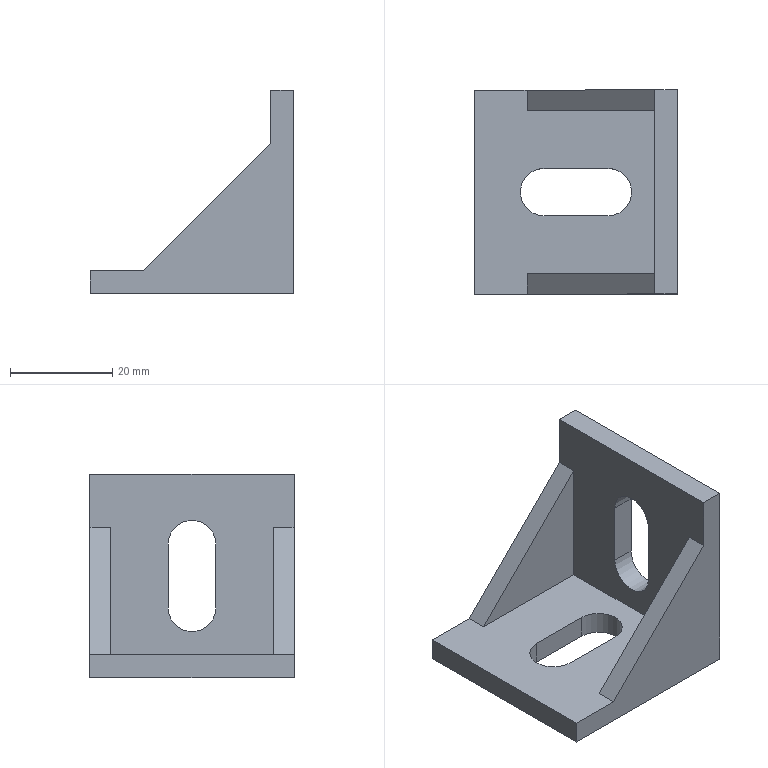Part | STEP file | 40x40 angle bracket | 1 solid | 20 faces | box 39.8 x 40 x 39.8 mm | volume 14360 mm3 | plane 16 | cylinder 4 | commonest cylinder face diameters 9.3 x4
STEP:
#1=CARTESIAN_POINT('',(0.,0.,0.));
#2=DIRECTION('',(0.,0.,1.));
#3=DIRECTION('',(1.,0.,0.));
#4=AXIS2_PLACEMENT_3D('',#1,#2,#3);
#5=CARTESIAN_POINT('',(400.35,-329.65,4.5));
#6=VERTEX_POINT('',#5);
#7=CARTESIAN_POINT('',(412.85,-329.65,4.5));
#8=VERTEX_POINT('',#7);
#9=CARTESIAN_POINT('',(386.7,-329.65,4.5));
#10=DIRECTION('',(1.,0.,0.));
#11=VECTOR('',#10,1.);
#12=LINE('',#9,#11);
#13=CARTESIAN_POINT('',(400.35,-329.65,44.5));
#14=DIRECTION('',(0.,-1.,0.));
#15=DIRECTION('',(0.,0.,1.));
#16=AXIS2_PLACEMENT_3D('',#13,#14,#15);
#17=PLANE('',#16);
#18=CARTESIAN_POINT('',(-40.,13.65));
#19=DIRECTION('',(0.,-1.));
#20=VECTOR('',#19,1.);
#21=LINE('',#18,#20);
#22=(GEOMETRIC_REPRESENTATION_CONTEXT(2)PARAMETRIC_REPRESENTATION_CONTEXT()REPRESENTATION_CONTEXT('',''));
#23=DEFINITIONAL_REPRESENTATION('',(#21),#22);
#24=PCURVE('',#17,#23);
#25=CARTESIAN_POINT('',(386.7,-305.,4.5));
#26=DIRECTION('',(0.,0.,1.));
#27=DIRECTION('',(1.,0.,0.));
#28=AXIS2_PLACEMENT_3D('',#25,#26,#27);
#29=PLANE('',#28);
#30=CARTESIAN_POINT('',(0.,-24.65));
#31=DIRECTION('',(1.,0.));
#32=VECTOR('',#31,1.);
#33=LINE('',#30,#32);
#34=(GEOMETRIC_REPRESENTATION_CONTEXT(2)PARAMETRIC_REPRESENTATION_CONTEXT()REPRESENTATION_CONTEXT('',''));
#35=DEFINITIONAL_REPRESENTATION('',(#33),#34);
#36=PCURVE('',#29,#35);
#37=SURFACE_CURVE('',#12,(#24,#36),.PCURVE_S1.);
#38=EDGE_CURVE('',#6,#8,#37,.T.);
#39=ORIENTED_EDGE('',*,*,#38,.T.);
#40=CARTESIAN_POINT('',(412.85,-329.65,0.));
#41=VERTEX_POINT('',#40);
#42=CARTESIAN_POINT('',(412.85,-329.65,44.5));
#43=DIRECTION('',(0.,0.,-1.));
#44=VECTOR('',#43,1.);
#45=LINE('',#42,#44);
#46=CARTESIAN_POINT('',(0.,-12.5));
#47=DIRECTION('',(-1.,0.));
#48=VECTOR('',#47,1.);
#49=LINE('',#46,#48);
#50=(GEOMETRIC_REPRESENTATION_CONTEXT(2)PARAMETRIC_REPRESENTATION_CONTEXT()REPRESENTATION_CONTEXT('',''));
#51=DEFINITIONAL_REPRESENTATION('',(#49),#50);
#52=PCURVE('',#17,#51);
#53=CARTESIAN_POINT('',(412.85,-325.,44.5));
#54=DIRECTION('',(0.,0.,-1.));
#55=DIRECTION('',(-1.,0.,0.));
#56=AXIS2_PLACEMENT_3D('',#53,#54,#55);
#57=CYLINDRICAL_SURFACE('',#56,4.65);
#58=CARTESIAN_POINT('',(4.712,0.));
#59=DIRECTION('',(0.,1.));
#60=VECTOR('',#59,1.);
#61=LINE('',#58,#60);
#62=(GEOMETRIC_REPRESENTATION_CONTEXT(2)PARAMETRIC_REPRESENTATION_CONTEXT()REPRESENTATION_CONTEXT('',''));
#63=DEFINITIONAL_REPRESENTATION('',(#61),#62);
#64=PCURVE('',#57,#63);
#65=SURFACE_CURVE('',#45,(#52,#64),.PCURVE_S1.);
#66=EDGE_CURVE('',#8,#41,#65,.T.);
#67=ORIENTED_EDGE('',*,*,#66,.T.);
#68=CARTESIAN_POINT('',(400.35,-329.65,0.));
#69=VERTEX_POINT('',#68);
#70=CARTESIAN_POINT('',(426.5,-329.65,0.));
#71=DIRECTION('',(-1.,0.,0.));
#72=VECTOR('',#71,1.);
#73=LINE('',#70,#72);
#74=CARTESIAN_POINT('',(-44.5,-26.15));
#75=DIRECTION('',(0.,1.));
#76=VECTOR('',#75,1.);
#77=LINE('',#74,#76);
#78=(GEOMETRIC_REPRESENTATION_CONTEXT(2)PARAMETRIC_REPRESENTATION_CONTEXT()REPRESENTATION_CONTEXT('',''));
#79=DEFINITIONAL_REPRESENTATION('',(#77),#78);
#80=PCURVE('',#17,#79);
#81=CARTESIAN_POINT('',(426.5,-305.,0.));
#82=DIRECTION('',(0.,0.,-1.));
#83=DIRECTION('',(-1.,0.,0.));
#84=AXIS2_PLACEMENT_3D('',#81,#82,#83);
#85=PLANE('',#84);
#86=CARTESIAN_POINT('',(0.,-24.65));
#87=DIRECTION('',(1.,0.));
#88=VECTOR('',#87,1.);
#89=LINE('',#86,#88);
#90=(GEOMETRIC_REPRESENTATION_CONTEXT(2)PARAMETRIC_REPRESENTATION_CONTEXT()REPRESENTATION_CONTEXT('',''));
#91=DEFINITIONAL_REPRESENTATION('',(#89),#90);
#92=PCURVE('',#85,#91);
#93=SURFACE_CURVE('',#73,(#80,#92),.PCURVE_S1.);
#94=EDGE_CURVE('',#41,#69,#93,.T.);
#95=ORIENTED_EDGE('',*,*,#94,.T.);
#96=CARTESIAN_POINT('',(400.35,-329.65,44.5));
#97=DIRECTION('',(0.,0.,-1.));
#98=VECTOR('',#97,1.);
#99=LINE('',#96,#98);
#100=CARTESIAN_POINT('',(0.,0.));
#101=DIRECTION('',(-1.,0.));
#102=VECTOR('',#101,1.);
#103=LINE('',#100,#102);
#104=(GEOMETRIC_REPRESENTATION_CONTEXT(2)PARAMETRIC_REPRESENTATION_CONTEXT()REPRESENTATION_CONTEXT('',''));
#105=DEFINITIONAL_REPRESENTATION('',(#103),#104);
#106=PCURVE('',#17,#105);
#107=CARTESIAN_POINT('',(400.35,-325.,44.5));
#108=DIRECTION('',(0.,0.,-1.));
#109=DIRECTION('',(-1.,0.,0.));
#110=AXIS2_PLACEMENT_3D('',#107,#108,#109);
#111=CYLINDRICAL_SURFACE('',#110,4.65);
#112=CARTESIAN_POINT('',(-1.571,0.));
#113=DIRECTION('',(0.,1.));
#114=VECTOR('',#113,1.);
#115=LINE('',#112,#114);
#116=(GEOMETRIC_REPRESENTATION_CONTEXT(2)PARAMETRIC_REPRESENTATION_CONTEXT()REPRESENTATION_CONTEXT('',''));
#117=DEFINITIONAL_REPRESENTATION('',(#115),#116);
#118=PCURVE('',#111,#117);
#119=SURFACE_CURVE('',#99,(#106,#118),.PCURVE_S1.);
#120=EDGE_CURVE('',#6,#69,#119,.T.);
#121=ORIENTED_EDGE('',*,*,#120,.F.);
#122=EDGE_LOOP('',(#39,#67,#95,#121));
#123=FACE_BOUND('',#122,.T.);
#124=ADVANCED_FACE('',(#123),#17,.F.);
#125=ORIENTED_EDGE('',*,*,#66,.T.);
#126=CARTESIAN_POINT('',(412.85,-320.35,0.));
#127=VERTEX_POINT('',#126);
#128=CARTESIAN_POINT('',(412.85,-325.,0.));
#129=DIRECTION('',(0.,0.,-1.));
#130=DIRECTION('',(-1.,0.,0.));
#131=AXIS2_PLACEMENT_3D('',#128,#129,#130);
#132=CIRCLE('',#131,4.65);
#133=CARTESIAN_POINT('',(0.,44.5));
#134=DIRECTION('',(1.,0.));
#135=VECTOR('',#134,1.);
#136=LINE('',#133,#135);
#137=(GEOMETRIC_REPRESENTATION_CONTEXT(2)PARAMETRIC_REPRESENTATION_CONTEXT()REPRESENTATION_CONTEXT('',''));
#138=DEFINITIONAL_REPRESENTATION('',(#136),#137);
#139=PCURVE('',#57,#138);
#140=CARTESIAN_POINT('',(13.65,-20.));
#141=DIRECTION('',(1.,0.));
#142=AXIS2_PLACEMENT_2D('',#140,#141);
#143=CIRCLE('',#142,4.65);
#144=(GEOMETRIC_REPRESENTATION_CONTEXT(2)PARAMETRIC_REPRESENTATION_CONTEXT()REPRESENTATION_CONTEXT('',''));
#145=DEFINITIONAL_REPRESENTATION('',(#143),#144);
#146=PCURVE('',#85,#145);
#147=SURFACE_CURVE('',#132,(#139,#146),.PCURVE_S1.);
#148=EDGE_CURVE('',#127,#41,#147,.T.);
#149=ORIENTED_EDGE('',*,*,#148,.F.);
#150=CARTESIAN_POINT('',(412.85,-320.35,4.5));
#151=VERTEX_POINT('',#150);
#152=CARTESIAN_POINT('',(412.85,-320.35,44.5));
#153=DIRECTION('',(0.,0.,-1.));
#154=VECTOR('',#153,1.);
#155=LINE('',#152,#154);
#156=CARTESIAN_POINT('',(1.571,0.));
#157=DIRECTION('',(0.,1.));
#158=VECTOR('',#157,1.);
#159=LINE('',#156,#158);
#160=(GEOMETRIC_REPRESENTATION_CONTEXT(2)PARAMETRIC_REPRESENTATION_CONTEXT()REPRESENTATION_CONTEXT('',''));
#161=DEFINITIONAL_REPRESENTATION('',(#159),#160);
#162=PCURVE('',#57,#161);
#163=CARTESIAN_POINT('',(412.85,-320.35,44.5));
#164=DIRECTION('',(0.,1.,0.));
#165=DIRECTION('',(0.,0.,-1.));
#166=AXIS2_PLACEMENT_3D('',#163,#164,#165);
#167=PLANE('',#166);
#168=CARTESIAN_POINT('',(0.,0.));
#169=DIRECTION('',(1.,0.));
#170=VECTOR('',#169,1.);
#171=LINE('',#168,#170);
#172=(GEOMETRIC_REPRESENTATION_CONTEXT(2)PARAMETRIC_REPRESENTATION_CONTEXT()REPRESENTATION_CONTEXT('',''));
#173=DEFINITIONAL_REPRESENTATION('',(#171),#172);
#174=PCURVE('',#167,#173);
#175=SURFACE_CURVE('',#155,(#162,#174),.PCURVE_S1.);
#176=EDGE_CURVE('',#151,#127,#175,.T.);
#177=ORIENTED_EDGE('',*,*,#176,.F.);
#178=CARTESIAN_POINT('',(412.85,-325.,4.5));
#179=DIRECTION('',(0.,0.,1.));
#180=DIRECTION('',(1.,0.,0.));
#181=AXIS2_PLACEMENT_3D('',#178,#179,#180);
#182=CIRCLE('',#181,4.65);
#183=CARTESIAN_POINT('',(9.425,40.));
#184=DIRECTION('',(-1.,0.));
#185=VECTOR('',#184,1.);
#186=LINE('',#183,#185);
#187=(GEOMETRIC_REPRESENTATION_CONTEXT(2)PARAMETRIC_REPRESENTATION_CONTEXT()REPRESENTATION_CONTEXT('',''));
#188=DEFINITIONAL_REPRESENTATION('',(#186),#187);
#189=PCURVE('',#57,#188);
#190=CARTESIAN_POINT('',(26.15,-20.));
#191=DIRECTION('',(1.,0.));
#192=AXIS2_PLACEMENT_2D('',#190,#191);
#193=CIRCLE('',#192,4.65);
#194=(GEOMETRIC_REPRESENTATION_CONTEXT(2)PARAMETRIC_REPRESENTATION_CONTEXT()REPRESENTATION_CONTEXT('',''));
#195=DEFINITIONAL_REPRESENTATION('',(#193),#194);
#196=PCURVE('',#29,#195);
#197=SURFACE_CURVE('',#182,(#189,#196),.PCURVE_S1.);
#198=EDGE_CURVE('',#8,#151,#197,.T.);
#199=ORIENTED_EDGE('',*,*,#198,.F.);
#200=EDGE_LOOP('',(#125,#149,#177,#199));
#201=FACE_BOUND('',#200,.F.);
#202=ADVANCED_FACE('',(#201),#57,.F.);
#203=CARTESIAN_POINT('',(400.35,-320.35,4.5));
#204=VERTEX_POINT('',#203);
#205=CARTESIAN_POINT('',(386.7,-320.35,4.5));
#206=DIRECTION('',(-1.,0.,0.));
#207=VECTOR('',#206,1.);
#208=LINE('',#205,#207);
#209=CARTESIAN_POINT('',(40.,26.15));
#210=DIRECTION('',(0.,1.));
#211=VECTOR('',#210,1.);
#212=LINE('',#209,#211);
#213=(GEOMETRIC_REPRESENTATION_CONTEXT(2)PARAMETRIC_REPRESENTATION_CONTEXT()REPRESENTATION_CONTEXT('',''));
#214=DEFINITIONAL_REPRESENTATION('',(#212),#213);
#215=PCURVE('',#167,#214);
#216=CARTESIAN_POINT('',(0.,-15.35));
#217=DIRECTION('',(-1.,0.));
#218=VECTOR('',#217,1.);
#219=LINE('',#216,#218);
#220=(GEOMETRIC_REPRESENTATION_CONTEXT(2)PARAMETRIC_REPRESENTATION_CONTEXT()REPRESENTATION_CONTEXT('',''));
#221=DEFINITIONAL_REPRESENTATION('',(#219),#220);
#222=PCURVE('',#29,#221);
#223=SURFACE_CURVE('',#208,(#215,#222),.PCURVE_S1.);
#224=EDGE_CURVE('',#151,#204,#223,.T.);
#225=ORIENTED_EDGE('',*,*,#224,.T.);
#226=CARTESIAN_POINT('',(400.35,-320.35,0.));
#227=VERTEX_POINT('',#226);
#228=CARTESIAN_POINT('',(400.35,-320.35,44.5));
#229=DIRECTION('',(0.,0.,-1.));
#230=VECTOR('',#229,1.);
#231=LINE('',#228,#230);
#232=CARTESIAN_POINT('',(0.,12.5));
#233=DIRECTION('',(1.,0.));
#234=VECTOR('',#233,1.);
#235=LINE('',#232,#234);
#236=(GEOMETRIC_REPRESENTATION_CONTEXT(2)PARAMETRIC_REPRESENTATION_CONTEXT()REPRESENTATION_CONTEXT('',''));
#237=DEFINITIONAL_REPRESENTATION('',(#235),#236);
#238=PCURVE('',#167,#237);
#239=CARTESIAN_POINT('',(1.571,0.));
#240=DIRECTION('',(0.,1.));
#241=VECTOR('',#240,1.);
#242=LINE('',#239,#241);
#243=(GEOMETRIC_REPRESENTATION_CONTEXT(2)PARAMETRIC_REPRESENTATION_CONTEXT()REPRESENTATION_CONTEXT('',''));
#244=DEFINITIONAL_REPRESENTATION('',(#242),#243);
#245=PCURVE('',#111,#244);
#246=SURFACE_CURVE('',#231,(#238,#245),.PCURVE_S1.);
#247=EDGE_CURVE('',#204,#227,#246,.T.);
#248=ORIENTED_EDGE('',*,*,#247,.T.);
#249=CARTESIAN_POINT('',(426.5,-320.35,0.));
#250=DIRECTION('',(1.,0.,0.));
#251=VECTOR('',#250,1.);
#252=LINE('',#249,#251);
#253=CARTESIAN_POINT('',(44.5,-13.65));
#254=DIRECTION('',(0.,-1.));
#255=VECTOR('',#254,1.);
#256=LINE('',#253,#255);
#257=(GEOMETRIC_REPRESENTATION_CONTEXT(2)PARAMETRIC_REPRESENTATION_CONTEXT()REPRESENTATION_CONTEXT('',''));
#258=DEFINITIONAL_REPRESENTATION('',(#256),#257);
#259=PCURVE('',#167,#258);
#260=CARTESIAN_POINT('',(0.,-15.35));
#261=DIRECTION('',(-1.,0.));
#262=VECTOR('',#261,1.);
#263=LINE('',#260,#262);
#264=(GEOMETRIC_REPRESENTATION_CONTEXT(2)PARAMETRIC_REPRESENTATION_CONTEXT()REPRESENTATION_CONTEXT('',''));
#265=DEFINITIONAL_REPRESENTATION('',(#263),#264);
#266=PCURVE('',#85,#265);
#267=SURFACE_CURVE('',#252,(#259,#266),.PCURVE_S1.);
#268=EDGE_CURVE('',#227,#127,#267,.T.);
#269=ORIENTED_EDGE('',*,*,#268,.T.);
#270=ORIENTED_EDGE('',*,*,#176,.F.);
#271=EDGE_LOOP('',(#225,#248,#269,#270));
#272=FACE_BOUND('',#271,.T.);
#273=ADVANCED_FACE('',(#272),#167,.F.);
#274=ORIENTED_EDGE('',*,*,#247,.T.);
#275=CARTESIAN_POINT('',(400.35,-325.,0.));
#276=DIRECTION('',(0.,0.,-1.));
#277=DIRECTION('',(-1.,0.,0.));
#278=AXIS2_PLACEMENT_3D('',#275,#276,#277);
#279=CIRCLE('',#278,4.65);
#280=CARTESIAN_POINT('',(-6.283,44.5));
#281=DIRECTION('',(1.,0.));
#282=VECTOR('',#281,1.);
#283=LINE('',#280,#282);
#284=(GEOMETRIC_REPRESENTATION_CONTEXT(2)PARAMETRIC_REPRESENTATION_CONTEXT()REPRESENTATION_CONTEXT('',''));
#285=DEFINITIONAL_REPRESENTATION('',(#283),#284);
#286=PCURVE('',#111,#285);
#287=CARTESIAN_POINT('',(26.15,-20.));
#288=DIRECTION('',(1.,0.));
#289=AXIS2_PLACEMENT_2D('',#287,#288);
#290=CIRCLE('',#289,4.65);
#291=(GEOMETRIC_REPRESENTATION_CONTEXT(2)PARAMETRIC_REPRESENTATION_CONTEXT()REPRESENTATION_CONTEXT('',''));
#292=DEFINITIONAL_REPRESENTATION('',(#290),#291);
#293=PCURVE('',#85,#292);
#294=SURFACE_CURVE('',#279,(#286,#293),.PCURVE_S1.);
#295=EDGE_CURVE('',#69,#227,#294,.T.);
#296=ORIENTED_EDGE('',*,*,#295,.F.);
#297=ORIENTED_EDGE('',*,*,#120,.F.);
#298=CARTESIAN_POINT('',(400.35,-325.,4.5));
#299=DIRECTION('',(0.,0.,1.));
#300=DIRECTION('',(1.,0.,0.));
#301=AXIS2_PLACEMENT_3D('',#298,#299,#300);
#302=CIRCLE('',#301,4.65);
#303=CARTESIAN_POINT('',(3.142,40.));
#304=DIRECTION('',(-1.,0.));
#305=VECTOR('',#304,1.);
#306=LINE('',#303,#305);
#307=(GEOMETRIC_REPRESENTATION_CONTEXT(2)PARAMETRIC_REPRESENTATION_CONTEXT()REPRESENTATION_CONTEXT('',''));
#308=DEFINITIONAL_REPRESENTATION('',(#306),#307);
#309=PCURVE('',#111,#308);
#310=CARTESIAN_POINT('',(13.65,-20.));
#311=DIRECTION('',(1.,0.));
#312=AXIS2_PLACEMENT_2D('',#310,#311);
#313=CIRCLE('',#312,4.65);
#314=(GEOMETRIC_REPRESENTATION_CONTEXT(2)PARAMETRIC_REPRESENTATION_CONTEXT()REPRESENTATION_CONTEXT('',''));
#315=DEFINITIONAL_REPRESENTATION('',(#313),#314);
#316=PCURVE('',#29,#315);
#317=SURFACE_CURVE('',#302,(#309,#316),.PCURVE_S1.);
#318=EDGE_CURVE('',#204,#6,#317,.T.);
#319=ORIENTED_EDGE('',*,*,#318,.F.);
#320=EDGE_LOOP('',(#274,#296,#297,#319));
#321=FACE_BOUND('',#320,.F.);
#322=ADVANCED_FACE('',(#321),#111,.F.);
#323=CARTESIAN_POINT('',(386.7,-345.,4.5));
#324=VERTEX_POINT('',#323);
#325=CARTESIAN_POINT('',(386.7,-345.,0.));
#326=VERTEX_POINT('',#325);
#327=CARTESIAN_POINT('',(386.7,-345.,0.));
#328=DIRECTION('',(0.,0.,-1.));
#329=VECTOR('',#328,1.);
#330=LINE('',#327,#329);
#331=CARTESIAN_POINT('',(386.7,-305.,0.));
#332=DIRECTION('',(-1.,0.,0.));
#333=DIRECTION('',(0.,0.,1.));
#334=AXIS2_PLACEMENT_3D('',#331,#332,#333);
#335=PLANE('',#334);
#336=CARTESIAN_POINT('',(0.,-40.));
#337=DIRECTION('',(-1.,0.));
#338=VECTOR('',#337,1.);
#339=LINE('',#336,#338);
#340=(GEOMETRIC_REPRESENTATION_CONTEXT(2)PARAMETRIC_REPRESENTATION_CONTEXT()REPRESENTATION_CONTEXT('',''));
#341=DEFINITIONAL_REPRESENTATION('',(#339),#340);
#342=PCURVE('',#335,#341);
#343=CARTESIAN_POINT('',(-13.5,-345.,0.));
#344=DIRECTION('',(0.,-1.,0.));
#345=DIRECTION('',(0.,0.,1.));
#346=AXIS2_PLACEMENT_3D('',#343,#344,#345);
#347=PLANE('',#346);
#348=CARTESIAN_POINT('',(0.,-400.2));
#349=DIRECTION('',(-1.,0.));
#350=VECTOR('',#349,1.);
#351=LINE('',#348,#350);
#352=(GEOMETRIC_REPRESENTATION_CONTEXT(2)PARAMETRIC_REPRESENTATION_CONTEXT()REPRESENTATION_CONTEXT('',''));
#353=DEFINITIONAL_REPRESENTATION('',(#351),#352);
#354=PCURVE('',#347,#353);
#355=SURFACE_CURVE('',#330,(#342,#354),.PCURVE_S1.);
#356=EDGE_CURVE('',#324,#326,#355,.T.);
#357=ORIENTED_EDGE('',*,*,#356,.F.);
#358=CARTESIAN_POINT('',(386.7,-305.,4.5));
#359=VERTEX_POINT('',#358);
#360=CARTESIAN_POINT('',(386.7,-305.,4.5));
#361=DIRECTION('',(0.,1.,0.));
#362=VECTOR('',#361,1.);
#363=LINE('',#360,#362);
#364=CARTESIAN_POINT('',(4.5,0.));
#365=DIRECTION('',(0.,1.));
#366=VECTOR('',#365,1.);
#367=LINE('',#364,#366);
#368=(GEOMETRIC_REPRESENTATION_CONTEXT(2)PARAMETRIC_REPRESENTATION_CONTEXT()REPRESENTATION_CONTEXT('',''));
#369=DEFINITIONAL_REPRESENTATION('',(#367),#368);
#370=PCURVE('',#335,#369);
#371=CARTESIAN_POINT('',(0.,0.));
#372=DIRECTION('',(0.,1.));
#373=VECTOR('',#372,1.);
#374=LINE('',#371,#373);
#375=(GEOMETRIC_REPRESENTATION_CONTEXT(2)PARAMETRIC_REPRESENTATION_CONTEXT()REPRESENTATION_CONTEXT('',''));
#376=DEFINITIONAL_REPRESENTATION('',(#374),#375);
#377=PCURVE('',#29,#376);
#378=SURFACE_CURVE('',#363,(#370,#377),.PCURVE_S1.);
#379=EDGE_CURVE('',#324,#359,#378,.T.);
#380=ORIENTED_EDGE('',*,*,#379,.T.);
#381=CARTESIAN_POINT('',(386.7,-305.,0.));
#382=VERTEX_POINT('',#381);
#383=CARTESIAN_POINT('',(386.7,-305.,0.));
#384=DIRECTION('',(0.,0.,-1.));
#385=VECTOR('',#384,1.);
#386=LINE('',#383,#385);
#387=CARTESIAN_POINT('',(0.,0.));
#388=DIRECTION('',(-1.,0.));
#389=VECTOR('',#388,1.);
#390=LINE('',#387,#389);
#391=(GEOMETRIC_REPRESENTATION_CONTEXT(2)PARAMETRIC_REPRESENTATION_CONTEXT()REPRESENTATION_CONTEXT('',''));
#392=DEFINITIONAL_REPRESENTATION('',(#390),#391);
#393=PCURVE('',#335,#392);
#394=CARTESIAN_POINT('',(-13.5,-305.,0.));
#395=DIRECTION('',(0.,-1.,0.));
#396=DIRECTION('',(0.,0.,1.));
#397=AXIS2_PLACEMENT_3D('',#394,#395,#396);
#398=PLANE('',#397);
#399=CARTESIAN_POINT('',(0.,-400.2));
#400=DIRECTION('',(-1.,0.));
#401=VECTOR('',#400,1.);
#402=LINE('',#399,#401);
#403=(GEOMETRIC_REPRESENTATION_CONTEXT(2)PARAMETRIC_REPRESENTATION_CONTEXT()REPRESENTATION_CONTEXT('',''));
#404=DEFINITIONAL_REPRESENTATION('',(#402),#403);
#405=PCURVE('',#398,#404);
#406=SURFACE_CURVE('',#386,(#393,#405),.PCURVE_S1.);
#407=EDGE_CURVE('',#359,#382,#406,.T.);
#408=ORIENTED_EDGE('',*,*,#407,.T.);
#409=CARTESIAN_POINT('',(386.7,-305.,0.));
#410=DIRECTION('',(0.,1.,0.));
#411=VECTOR('',#410,1.);
#412=LINE('',#409,#411);
#413=CARTESIAN_POINT('',(0.,0.));
#414=DIRECTION('',(0.,1.));
#415=VECTOR('',#414,1.);
#416=LINE('',#413,#415);
#417=(GEOMETRIC_REPRESENTATION_CONTEXT(2)PARAMETRIC_REPRESENTATION_CONTEXT()REPRESENTATION_CONTEXT('',''));
#418=DEFINITIONAL_REPRESENTATION('',(#416),#417);
#419=PCURVE('',#335,#418);
#420=CARTESIAN_POINT('',(39.8,0.));
#421=DIRECTION('',(0.,1.));
#422=VECTOR('',#421,1.);
#423=LINE('',#420,#422);
#424=(GEOMETRIC_REPRESENTATION_CONTEXT(2)PARAMETRIC_REPRESENTATION_CONTEXT()REPRESENTATION_CONTEXT('',''));
#425=DEFINITIONAL_REPRESENTATION('',(#423),#424);
#426=PCURVE('',#85,#425);
#427=SURFACE_CURVE('',#412,(#419,#426),.PCURVE_S1.);
#428=EDGE_CURVE('',#326,#382,#427,.T.);
#429=ORIENTED_EDGE('',*,*,#428,.F.);
#430=EDGE_LOOP('',(#357,#380,#408,#429));
#431=FACE_BOUND('',#430,.T.);
#432=ADVANCED_FACE('',(#431),#335,.T.);
#433=ORIENTED_EDGE('',*,*,#295,.F.);
#434=ORIENTED_EDGE('',*,*,#94,.F.);
#435=ORIENTED_EDGE('',*,*,#148,.F.);
#436=ORIENTED_EDGE('',*,*,#268,.F.);
#437=EDGE_LOOP('',(#433,#434,#435,#436));
#438=FACE_BOUND('',#437,.T.);
#439=CARTESIAN_POINT('',(426.5,-345.,0.));
#440=VERTEX_POINT('',#439);
#441=CARTESIAN_POINT('',(426.5,-345.,0.));
#442=DIRECTION('',(1.,0.,0.));
#443=VECTOR('',#442,1.);
#444=LINE('',#441,#443);
#445=CARTESIAN_POINT('',(0.,-40.));
#446=DIRECTION('',(-1.,0.));
#447=VECTOR('',#446,1.);
#448=LINE('',#445,#447);
#449=(GEOMETRIC_REPRESENTATION_CONTEXT(2)PARAMETRIC_REPRESENTATION_CONTEXT()REPRESENTATION_CONTEXT('',''));
#450=DEFINITIONAL_REPRESENTATION('',(#448),#449);
#451=PCURVE('',#85,#450);
#452=CARTESIAN_POINT('',(0.,-440.));
#453=DIRECTION('',(0.,-1.));
#454=VECTOR('',#453,1.);
#455=LINE('',#452,#454);
#456=(GEOMETRIC_REPRESENTATION_CONTEXT(2)PARAMETRIC_REPRESENTATION_CONTEXT()REPRESENTATION_CONTEXT('',''));
#457=DEFINITIONAL_REPRESENTATION('',(#455),#456);
#458=PCURVE('',#347,#457);
#459=SURFACE_CURVE('',#444,(#451,#458),.PCURVE_S1.);
#460=EDGE_CURVE('',#326,#440,#459,.T.);
#461=ORIENTED_EDGE('',*,*,#460,.F.);
#462=ORIENTED_EDGE('',*,*,#428,.T.);
#463=CARTESIAN_POINT('',(426.5,-305.,0.));
#464=VERTEX_POINT('',#463);
#465=CARTESIAN_POINT('',(426.5,-305.,0.));
#466=DIRECTION('',(1.,0.,0.));
#467=VECTOR('',#466,1.);
#468=LINE('',#465,#467);
#469=CARTESIAN_POINT('',(0.,0.));
#470=DIRECTION('',(-1.,0.));
#471=VECTOR('',#470,1.);
#472=LINE('',#469,#471);
#473=(GEOMETRIC_REPRESENTATION_CONTEXT(2)PARAMETRIC_REPRESENTATION_CONTEXT()REPRESENTATION_CONTEXT('',''));
#474=DEFINITIONAL_REPRESENTATION('',(#472),#473);
#475=PCURVE('',#85,#474);
#476=CARTESIAN_POINT('',(0.,-440.));
#477=DIRECTION('',(0.,-1.));
#478=VECTOR('',#477,1.);
#479=LINE('',#476,#478);
#480=(GEOMETRIC_REPRESENTATION_CONTEXT(2)PARAMETRIC_REPRESENTATION_CONTEXT()REPRESENTATION_CONTEXT('',''));
#481=DEFINITIONAL_REPRESENTATION('',(#479),#480);
#482=PCURVE('',#398,#481);
#483=SURFACE_CURVE('',#468,(#475,#482),.PCURVE_S1.);
#484=EDGE_CURVE('',#382,#464,#483,.T.);
#485=ORIENTED_EDGE('',*,*,#484,.T.);
#486=CARTESIAN_POINT('',(426.5,-305.,0.));
#487=DIRECTION('',(0.,1.,0.));
#488=VECTOR('',#487,1.);
#489=LINE('',#486,#488);
#490=CARTESIAN_POINT('',(0.,0.));
#491=DIRECTION('',(0.,1.));
#492=VECTOR('',#491,1.);
#493=LINE('',#490,#492);
#494=(GEOMETRIC_REPRESENTATION_CONTEXT(2)PARAMETRIC_REPRESENTATION_CONTEXT()REPRESENTATION_CONTEXT('',''));
#495=DEFINITIONAL_REPRESENTATION('',(#493),#494);
#496=PCURVE('',#85,#495);
#497=CARTESIAN_POINT('',(426.5,-305.,39.8));
#498=DIRECTION('',(1.,0.,0.));
#499=DIRECTION('',(0.,0.,-1.));
#500=AXIS2_PLACEMENT_3D('',#497,#498,#499);
#501=PLANE('',#500);
#502=CARTESIAN_POINT('',(39.8,0.));
#503=DIRECTION('',(0.,1.));
#504=VECTOR('',#503,1.);
#505=LINE('',#502,#504);
#506=(GEOMETRIC_REPRESENTATION_CONTEXT(2)PARAMETRIC_REPRESENTATION_CONTEXT()REPRESENTATION_CONTEXT('',''));
#507=DEFINITIONAL_REPRESENTATION('',(#505),#506);
#508=PCURVE('',#501,#507);
#509=SURFACE_CURVE('',#489,(#496,#508),.PCURVE_S1.);
#510=EDGE_CURVE('',#440,#464,#509,.T.);
#511=ORIENTED_EDGE('',*,*,#510,.F.);
#512=EDGE_LOOP('',(#461,#462,#485,#511));
#513=FACE_BOUND('',#512,.T.);
#514=ADVANCED_FACE('',(#438,#513),#85,.T.);
#515=ORIENTED_EDGE('',*,*,#407,.F.);
#516=CARTESIAN_POINT('',(397.,-305.,4.5));
#517=VERTEX_POINT('',#516);
#518=CARTESIAN_POINT('',(386.7,-305.,4.5));
#519=DIRECTION('',(-1.,0.,0.));
#520=VECTOR('',#519,1.);
#521=LINE('',#518,#520);
#522=CARTESIAN_POINT('',(4.5,-400.2));
#523=DIRECTION('',(0.,1.));
#524=VECTOR('',#523,1.);
#525=LINE('',#522,#524);
#526=(GEOMETRIC_REPRESENTATION_CONTEXT(2)PARAMETRIC_REPRESENTATION_CONTEXT()REPRESENTATION_CONTEXT('',''));
#527=DEFINITIONAL_REPRESENTATION('',(#525),#526);
#528=PCURVE('',#398,#527);
#529=CARTESIAN_POINT('',(0.,0.));
#530=DIRECTION('',(-1.,0.));
#531=VECTOR('',#530,1.);
#532=LINE('',#529,#531);
#533=(GEOMETRIC_REPRESENTATION_CONTEXT(2)PARAMETRIC_REPRESENTATION_CONTEXT()REPRESENTATION_CONTEXT('',''));
#534=DEFINITIONAL_REPRESENTATION('',(#532),#533);
#535=PCURVE('',#29,#534);
#536=SURFACE_CURVE('',#521,(#528,#535),.PCURVE_S1.);
#537=EDGE_CURVE('',#517,#359,#536,.T.);
#538=ORIENTED_EDGE('',*,*,#537,.F.);
#539=CARTESIAN_POINT('',(422.,-305.,29.5));
#540=VERTEX_POINT('',#539);
#541=CARTESIAN_POINT('',(189.5,-305.,-203.));
#542=DIRECTION('',(0.7071,0.,0.7071));
#543=VECTOR('',#542,1.);
#544=LINE('',#541,#543);
#545=CARTESIAN_POINT('',(-203.,-203.));
#546=DIRECTION('',(0.7071,-0.7071));
#547=VECTOR('',#546,1.);
#548=LINE('',#545,#547);
#549=(GEOMETRIC_REPRESENTATION_CONTEXT(2)PARAMETRIC_REPRESENTATION_CONTEXT()REPRESENTATION_CONTEXT('',''));
#550=DEFINITIONAL_REPRESENTATION('',(#548),#549);
#551=PCURVE('',#398,#550);
#552=CARTESIAN_POINT('',(397.,-305.,4.5));
#553=DIRECTION('',(-0.7071,0.,0.7071));
#554=DIRECTION('',(0.,1.,0.));
#555=AXIS2_PLACEMENT_3D('',#552,#553,#554);
#556=PLANE('',#555);
#557=CARTESIAN_POINT('',(0.,293.449));
#558=DIRECTION('',(0.,-1.));
#559=VECTOR('',#558,1.);
#560=LINE('',#557,#559);
#561=(GEOMETRIC_REPRESENTATION_CONTEXT(2)PARAMETRIC_REPRESENTATION_CONTEXT()REPRESENTATION_CONTEXT('',''));
#562=DEFINITIONAL_REPRESENTATION('',(#560),#561);
#563=PCURVE('',#556,#562);
#564=SURFACE_CURVE('',#544,(#551,#563),.PCURVE_S1.);
#565=EDGE_CURVE('',#517,#540,#564,.T.);
#566=ORIENTED_EDGE('',*,*,#565,.T.);
#567=CARTESIAN_POINT('',(422.,-305.,39.8));
#568=VERTEX_POINT('',#567);
#569=CARTESIAN_POINT('',(422.,-305.,4.5));
#570=DIRECTION('',(0.,0.,-1.));
#571=VECTOR('',#570,1.);
#572=LINE('',#569,#571);
#573=CARTESIAN_POINT('',(4.5,-435.5));
#574=DIRECTION('',(-1.,0.));
#575=VECTOR('',#574,1.);
#576=LINE('',#573,#575);
#577=(GEOMETRIC_REPRESENTATION_CONTEXT(2)PARAMETRIC_REPRESENTATION_CONTEXT()REPRESENTATION_CONTEXT('',''));
#578=DEFINITIONAL_REPRESENTATION('',(#576),#577);
#579=PCURVE('',#398,#578);
#580=CARTESIAN_POINT('',(422.,-305.,4.5));
#581=DIRECTION('',(-1.,0.,0.));
#582=DIRECTION('',(0.,0.,1.));
#583=AXIS2_PLACEMENT_3D('',#580,#581,#582);
#584=PLANE('',#583);
#585=CARTESIAN_POINT('',(0.,0.));
#586=DIRECTION('',(-1.,0.));
#587=VECTOR('',#586,1.);
#588=LINE('',#585,#587);
#589=(GEOMETRIC_REPRESENTATION_CONTEXT(2)PARAMETRIC_REPRESENTATION_CONTEXT()REPRESENTATION_CONTEXT('',''));
#590=DEFINITIONAL_REPRESENTATION('',(#588),#589);
#591=PCURVE('',#584,#590);
#592=SURFACE_CURVE('',#572,(#579,#591),.PCURVE_S1.);
#593=EDGE_CURVE('',#568,#540,#592,.T.);
#594=ORIENTED_EDGE('',*,*,#593,.F.);
#595=CARTESIAN_POINT('',(426.5,-305.,39.8));
#596=VERTEX_POINT('',#595);
#597=CARTESIAN_POINT('',(422.,-305.,39.8));
#598=DIRECTION('',(-1.,0.,0.));
#599=VECTOR('',#598,1.);
#600=LINE('',#597,#599);
#601=CARTESIAN_POINT('',(39.8,-435.5));
#602=DIRECTION('',(0.,1.));
#603=VECTOR('',#602,1.);
#604=LINE('',#601,#603);
#605=(GEOMETRIC_REPRESENTATION_CONTEXT(2)PARAMETRIC_REPRESENTATION_CONTEXT()REPRESENTATION_CONTEXT('',''));
#606=DEFINITIONAL_REPRESENTATION('',(#604),#605);
#607=PCURVE('',#398,#606);
#608=CARTESIAN_POINT('',(422.,-305.,39.8));
#609=DIRECTION('',(0.,0.,1.));
#610=DIRECTION('',(1.,0.,0.));
#611=AXIS2_PLACEMENT_3D('',#608,#609,#610);
#612=PLANE('',#611);
#613=CARTESIAN_POINT('',(0.,0.));
#614=DIRECTION('',(-1.,0.));
#615=VECTOR('',#614,1.);
#616=LINE('',#613,#615);
#617=(GEOMETRIC_REPRESENTATION_CONTEXT(2)PARAMETRIC_REPRESENTATION_CONTEXT()REPRESENTATION_CONTEXT('',''));
#618=DEFINITIONAL_REPRESENTATION('',(#616),#617);
#619=PCURVE('',#612,#618);
#620=SURFACE_CURVE('',#600,(#607,#619),.PCURVE_S1.);
#621=EDGE_CURVE('',#596,#568,#620,.T.);
#622=ORIENTED_EDGE('',*,*,#621,.F.);
#623=CARTESIAN_POINT('',(426.5,-305.,39.8));
#624=DIRECTION('',(0.,0.,1.));
#625=VECTOR('',#624,1.);
#626=LINE('',#623,#625);
#627=CARTESIAN_POINT('',(39.8,-440.));
#628=DIRECTION('',(1.,0.));
#629=VECTOR('',#628,1.);
#630=LINE('',#627,#629);
#631=(GEOMETRIC_REPRESENTATION_CONTEXT(2)PARAMETRIC_REPRESENTATION_CONTEXT()REPRESENTATION_CONTEXT('',''));
#632=DEFINITIONAL_REPRESENTATION('',(#630),#631);
#633=PCURVE('',#398,#632);
#634=CARTESIAN_POINT('',(0.,0.));
#635=DIRECTION('',(-1.,0.));
#636=VECTOR('',#635,1.);
#637=LINE('',#634,#636);
#638=(GEOMETRIC_REPRESENTATION_CONTEXT(2)PARAMETRIC_REPRESENTATION_CONTEXT()REPRESENTATION_CONTEXT('',''));
#639=DEFINITIONAL_REPRESENTATION('',(#637),#638);
#640=PCURVE('',#501,#639);
#641=SURFACE_CURVE('',#626,(#633,#640),.PCURVE_S1.);
#642=EDGE_CURVE('',#464,#596,#641,.T.);
#643=ORIENTED_EDGE('',*,*,#642,.F.);
#644=ORIENTED_EDGE('',*,*,#484,.F.);
#645=EDGE_LOOP('',(#515,#538,#566,#594,#622,#643,#644));
#646=FACE_BOUND('',#645,.T.);
#647=ADVANCED_FACE('',(#646),#398,.F.);
#648=CARTESIAN_POINT('',(426.5,-345.,39.8));
#649=VERTEX_POINT('',#648);
#650=CARTESIAN_POINT('',(422.,-345.,39.8));
#651=VERTEX_POINT('',#650);
#652=CARTESIAN_POINT('',(422.,-345.,39.8));
#653=DIRECTION('',(-1.,0.,0.));
#654=VECTOR('',#653,1.);
#655=LINE('',#652,#654);
#656=CARTESIAN_POINT('',(0.,-40.));
#657=DIRECTION('',(-1.,0.));
#658=VECTOR('',#657,1.);
#659=LINE('',#656,#658);
#660=(GEOMETRIC_REPRESENTATION_CONTEXT(2)PARAMETRIC_REPRESENTATION_CONTEXT()REPRESENTATION_CONTEXT('',''));
#661=DEFINITIONAL_REPRESENTATION('',(#659),#660);
#662=PCURVE('',#612,#661);
#663=CARTESIAN_POINT('',(39.8,-435.5));
#664=DIRECTION('',(0.,1.));
#665=VECTOR('',#664,1.);
#666=LINE('',#663,#665);
#667=(GEOMETRIC_REPRESENTATION_CONTEXT(2)PARAMETRIC_REPRESENTATION_CONTEXT()REPRESENTATION_CONTEXT('',''));
#668=DEFINITIONAL_REPRESENTATION('',(#666),#667);
#669=PCURVE('',#347,#668);
#670=SURFACE_CURVE('',#655,(#662,#669),.PCURVE_S1.);
#671=EDGE_CURVE('',#649,#651,#670,.T.);
#672=ORIENTED_EDGE('',*,*,#671,.F.);
#673=CARTESIAN_POINT('',(426.5,-305.,39.8));
#674=DIRECTION('',(0.,1.,0.));
#675=VECTOR('',#674,1.);
#676=LINE('',#673,#675);
#677=CARTESIAN_POINT('',(4.5,0.));
#678=DIRECTION('',(0.,1.));
#679=VECTOR('',#678,1.);
#680=LINE('',#677,#679);
#681=(GEOMETRIC_REPRESENTATION_CONTEXT(2)PARAMETRIC_REPRESENTATION_CONTEXT()REPRESENTATION_CONTEXT('',''));
#682=DEFINITIONAL_REPRESENTATION('',(#680),#681);
#683=PCURVE('',#612,#682);
#684=CARTESIAN_POINT('',(0.,0.));
#685=DIRECTION('',(0.,1.));
#686=VECTOR('',#685,1.);
#687=LINE('',#684,#686);
#688=(GEOMETRIC_REPRESENTATION_CONTEXT(2)PARAMETRIC_REPRESENTATION_CONTEXT()REPRESENTATION_CONTEXT('',''));
#689=DEFINITIONAL_REPRESENTATION('',(#687),#688);
#690=PCURVE('',#501,#689);
#691=SURFACE_CURVE('',#676,(#683,#690),.PCURVE_S1.);
#692=EDGE_CURVE('',#649,#596,#691,.T.);
#693=ORIENTED_EDGE('',*,*,#692,.T.);
#694=ORIENTED_EDGE('',*,*,#621,.T.);
#695=CARTESIAN_POINT('',(422.,-305.,39.8));
#696=DIRECTION('',(0.,1.,0.));
#697=VECTOR('',#696,1.);
#698=LINE('',#695,#697);
#699=CARTESIAN_POINT('',(0.,0.));
#700=DIRECTION('',(0.,1.));
#701=VECTOR('',#700,1.);
#702=LINE('',#699,#701);
#703=(GEOMETRIC_REPRESENTATION_CONTEXT(2)PARAMETRIC_REPRESENTATION_CONTEXT()REPRESENTATION_CONTEXT('',''));
#704=DEFINITIONAL_REPRESENTATION('',(#702),#703);
#705=PCURVE('',#612,#704);
#706=CARTESIAN_POINT('',(35.3,0.));
#707=DIRECTION('',(0.,1.));
#708=VECTOR('',#707,1.);
#709=LINE('',#706,#708);
#710=(GEOMETRIC_REPRESENTATION_CONTEXT(2)PARAMETRIC_REPRESENTATION_CONTEXT()REPRESENTATION_CONTEXT('',''));
#711=DEFINITIONAL_REPRESENTATION('',(#709),#710);
#712=PCURVE('',#584,#711);
#713=SURFACE_CURVE('',#698,(#705,#712),.PCURVE_S1.);
#714=EDGE_CURVE('',#651,#568,#713,.T.);
#715=ORIENTED_EDGE('',*,*,#714,.F.);
#716=EDGE_LOOP('',(#672,#693,#694,#715));
#717=FACE_BOUND('',#716,.T.);
#718=ADVANCED_FACE('',(#717),#612,.T.);
#719=ORIENTED_EDGE('',*,*,#356,.T.);
#720=ORIENTED_EDGE('',*,*,#460,.T.);
#721=CARTESIAN_POINT('',(426.5,-345.,39.8));
#722=DIRECTION('',(0.,0.,1.));
#723=VECTOR('',#722,1.);
#724=LINE('',#721,#723);
#725=CARTESIAN_POINT('',(39.8,-440.));
#726=DIRECTION('',(1.,0.));
#727=VECTOR('',#726,1.);
#728=LINE('',#725,#727);
#729=(GEOMETRIC_REPRESENTATION_CONTEXT(2)PARAMETRIC_REPRESENTATION_CONTEXT()REPRESENTATION_CONTEXT('',''));
#730=DEFINITIONAL_REPRESENTATION('',(#728),#729);
#731=PCURVE('',#347,#730);
#732=CARTESIAN_POINT('',(0.,-40.));
#733=DIRECTION('',(-1.,0.));
#734=VECTOR('',#733,1.);
#735=LINE('',#732,#734);
#736=(GEOMETRIC_REPRESENTATION_CONTEXT(2)PARAMETRIC_REPRESENTATION_CONTEXT()REPRESENTATION_CONTEXT('',''));
#737=DEFINITIONAL_REPRESENTATION('',(#735),#736);
#738=PCURVE('',#501,#737);
#739=SURFACE_CURVE('',#724,(#731,#738),.PCURVE_S1.);
#740=EDGE_CURVE('',#440,#649,#739,.T.);
#741=ORIENTED_EDGE('',*,*,#740,.T.);
#742=ORIENTED_EDGE('',*,*,#671,.T.);
#743=CARTESIAN_POINT('',(422.,-345.,29.5));
#744=VERTEX_POINT('',#743);
#745=CARTESIAN_POINT('',(422.,-345.,4.5));
#746=DIRECTION('',(0.,0.,-1.));
#747=VECTOR('',#746,1.);
#748=LINE('',#745,#747);
#749=CARTESIAN_POINT('',(4.5,-435.5));
#750=DIRECTION('',(-1.,0.));
#751=VECTOR('',#750,1.);
#752=LINE('',#749,#751);
#753=(GEOMETRIC_REPRESENTATION_CONTEXT(2)PARAMETRIC_REPRESENTATION_CONTEXT()REPRESENTATION_CONTEXT('',''));
#754=DEFINITIONAL_REPRESENTATION('',(#752),#753);
#755=PCURVE('',#347,#754);
#756=CARTESIAN_POINT('',(0.,-40.));
#757=DIRECTION('',(-1.,0.));
#758=VECTOR('',#757,1.);
#759=LINE('',#756,#758);
#760=(GEOMETRIC_REPRESENTATION_CONTEXT(2)PARAMETRIC_REPRESENTATION_CONTEXT()REPRESENTATION_CONTEXT('',''));
#761=DEFINITIONAL_REPRESENTATION('',(#759),#760);
#762=PCURVE('',#584,#761);
#763=SURFACE_CURVE('',#748,(#755,#762),.PCURVE_S1.);
#764=EDGE_CURVE('',#651,#744,#763,.T.);
#765=ORIENTED_EDGE('',*,*,#764,.T.);
#766=CARTESIAN_POINT('',(397.,-345.,4.5));
#767=VERTEX_POINT('',#766);
#768=CARTESIAN_POINT('',(397.,-345.,4.5));
#769=DIRECTION('',(-0.7071,0.,-0.7071));
#770=VECTOR('',#769,1.);
#771=LINE('',#768,#770);
#772=CARTESIAN_POINT('',(4.5,-410.5));
#773=DIRECTION('',(-0.7071,0.7071));
#774=VECTOR('',#773,1.);
#775=LINE('',#772,#774);
#776=(GEOMETRIC_REPRESENTATION_CONTEXT(2)PARAMETRIC_REPRESENTATION_CONTEXT()REPRESENTATION_CONTEXT('',''));
#777=DEFINITIONAL_REPRESENTATION('',(#775),#776);
#778=PCURVE('',#347,#777);
#779=CARTESIAN_POINT('',(397.,-305.,4.5));
#780=DIRECTION('',(-0.7071,0.,0.7071));
#781=DIRECTION('',(0.,1.,0.));
#782=AXIS2_PLACEMENT_3D('',#779,#780,#781);
#783=PLANE('',#782);
#784=CARTESIAN_POINT('',(-40.,0.));
#785=DIRECTION('',(0.,1.));
#786=VECTOR('',#785,1.);
#787=LINE('',#784,#786);
#788=(GEOMETRIC_REPRESENTATION_CONTEXT(2)PARAMETRIC_REPRESENTATION_CONTEXT()REPRESENTATION_CONTEXT('',''));
#789=DEFINITIONAL_REPRESENTATION('',(#787),#788);
#790=PCURVE('',#783,#789);
#791=SURFACE_CURVE('',#771,(#778,#790),.PCURVE_S1.);
#792=EDGE_CURVE('',#744,#767,#791,.T.);
#793=ORIENTED_EDGE('',*,*,#792,.T.);
#794=CARTESIAN_POINT('',(386.7,-345.,4.5));
#795=DIRECTION('',(-1.,0.,0.));
#796=VECTOR('',#795,1.);
#797=LINE('',#794,#796);
#798=CARTESIAN_POINT('',(4.5,-400.2));
#799=DIRECTION('',(0.,1.));
#800=VECTOR('',#799,1.);
#801=LINE('',#798,#800);
#802=(GEOMETRIC_REPRESENTATION_CONTEXT(2)PARAMETRIC_REPRESENTATION_CONTEXT()REPRESENTATION_CONTEXT('',''));
#803=DEFINITIONAL_REPRESENTATION('',(#801),#802);
#804=PCURVE('',#347,#803);
#805=CARTESIAN_POINT('',(0.,-40.));
#806=DIRECTION('',(-1.,0.));
#807=VECTOR('',#806,1.);
#808=LINE('',#805,#807);
#809=(GEOMETRIC_REPRESENTATION_CONTEXT(2)PARAMETRIC_REPRESENTATION_CONTEXT()REPRESENTATION_CONTEXT('',''));
#810=DEFINITIONAL_REPRESENTATION('',(#808),#809);
#811=PCURVE('',#29,#810);
#812=SURFACE_CURVE('',#797,(#804,#811),.PCURVE_S1.);
#813=EDGE_CURVE('',#767,#324,#812,.T.);
#814=ORIENTED_EDGE('',*,*,#813,.T.);
#815=EDGE_LOOP('',(#719,#720,#741,#742,#765,#793,#814));
#816=FACE_BOUND('',#815,.T.);
#817=ADVANCED_FACE('',(#816),#347,.T.);
#818=CARTESIAN_POINT('',(426.5,-320.35,13.65));
#819=VERTEX_POINT('',#818);
#820=CARTESIAN_POINT('',(426.5,-320.35,26.15));
#821=VERTEX_POINT('',#820);
#822=CARTESIAN_POINT('',(426.5,-320.35,39.8));
#823=DIRECTION('',(0.,0.,1.));
#824=VECTOR('',#823,1.);
#825=LINE('',#822,#824);
#826=CARTESIAN_POINT('',(0.,-15.35));
#827=DIRECTION('',(-1.,0.));
#828=VECTOR('',#827,1.);
#829=LINE('',#826,#828);
#830=(GEOMETRIC_REPRESENTATION_CONTEXT(2)PARAMETRIC_REPRESENTATION_CONTEXT()REPRESENTATION_CONTEXT('',''));
#831=DEFINITIONAL_REPRESENTATION('',(#829),#830);
#832=PCURVE('',#501,#831);
#833=CARTESIAN_POINT('',(382.,-320.35,13.65));
#834=DIRECTION('',(0.,1.,0.));
#835=DIRECTION('',(1.,0.,0.));
#836=AXIS2_PLACEMENT_3D('',#833,#834,#835);
#837=PLANE('',#836);
#838=CARTESIAN_POINT('',(44.5,-26.15));
#839=DIRECTION('',(0.,-1.));
#840=VECTOR('',#839,1.);
#841=LINE('',#838,#840);
#842=(GEOMETRIC_REPRESENTATION_CONTEXT(2)PARAMETRIC_REPRESENTATION_CONTEXT()REPRESENTATION_CONTEXT('',''));
#843=DEFINITIONAL_REPRESENTATION('',(#841),#842);
#844=PCURVE('',#837,#843);
#845=SURFACE_CURVE('',#825,(#832,#844),.PCURVE_S1.);
#846=EDGE_CURVE('',#819,#821,#845,.T.);
#847=ORIENTED_EDGE('',*,*,#846,.F.);
#848=CARTESIAN_POINT('',(426.5,-329.65,13.65));
#849=VERTEX_POINT('',#848);
#850=CARTESIAN_POINT('',(426.5,-325.,13.65));
#851=DIRECTION('',(1.,0.,0.));
#852=DIRECTION('',(0.,0.,-1.));
#853=AXIS2_PLACEMENT_3D('',#850,#851,#852);
#854=CIRCLE('',#853,4.65);
#855=CARTESIAN_POINT('',(26.15,-20.));
#856=DIRECTION('',(1.,0.));
#857=AXIS2_PLACEMENT_2D('',#855,#856);
#858=CIRCLE('',#857,4.65);
#859=(GEOMETRIC_REPRESENTATION_CONTEXT(2)PARAMETRIC_REPRESENTATION_CONTEXT()REPRESENTATION_CONTEXT('',''));
#860=DEFINITIONAL_REPRESENTATION('',(#858),#859);
#861=PCURVE('',#501,#860);
#862=CARTESIAN_POINT('',(382.,-325.,13.65));
#863=DIRECTION('',(1.,0.,0.));
#864=DIRECTION('',(0.,0.,1.));
#865=AXIS2_PLACEMENT_3D('',#862,#863,#864);
#866=CYLINDRICAL_SURFACE('',#865,4.65);
#867=CARTESIAN_POINT('',(-3.142,44.5));
#868=DIRECTION('',(1.,0.));
#869=VECTOR('',#868,1.);
#870=LINE('',#867,#869);
#871=(GEOMETRIC_REPRESENTATION_CONTEXT(2)PARAMETRIC_REPRESENTATION_CONTEXT()REPRESENTATION_CONTEXT('',''));
#872=DEFINITIONAL_REPRESENTATION('',(#870),#871);
#873=PCURVE('',#866,#872);
#874=SURFACE_CURVE('',#854,(#861,#873),.PCURVE_S1.);
#875=EDGE_CURVE('',#849,#819,#874,.T.);
#876=ORIENTED_EDGE('',*,*,#875,.F.);
#877=CARTESIAN_POINT('',(426.5,-329.65,26.15));
#878=VERTEX_POINT('',#877);
#879=CARTESIAN_POINT('',(426.5,-329.65,39.8));
#880=DIRECTION('',(0.,0.,-1.));
#881=VECTOR('',#880,1.);
#882=LINE('',#879,#881);
#883=CARTESIAN_POINT('',(0.,-24.65));
#884=DIRECTION('',(1.,0.));
#885=VECTOR('',#884,1.);
#886=LINE('',#883,#885);
#887=(GEOMETRIC_REPRESENTATION_CONTEXT(2)PARAMETRIC_REPRESENTATION_CONTEXT()REPRESENTATION_CONTEXT('',''));
#888=DEFINITIONAL_REPRESENTATION('',(#886),#887);
#889=PCURVE('',#501,#888);
#890=CARTESIAN_POINT('',(382.,-329.65,26.15));
#891=DIRECTION('',(0.,-1.,0.));
#892=DIRECTION('',(-1.,0.,0.));
#893=AXIS2_PLACEMENT_3D('',#890,#891,#892);
#894=PLANE('',#893);
#895=CARTESIAN_POINT('',(-44.5,-13.65));
#896=DIRECTION('',(0.,1.));
#897=VECTOR('',#896,1.);
#898=LINE('',#895,#897);
#899=(GEOMETRIC_REPRESENTATION_CONTEXT(2)PARAMETRIC_REPRESENTATION_CONTEXT()REPRESENTATION_CONTEXT('',''));
#900=DEFINITIONAL_REPRESENTATION('',(#898),#899);
#901=PCURVE('',#894,#900);
#902=SURFACE_CURVE('',#882,(#889,#901),.PCURVE_S1.);
#903=EDGE_CURVE('',#878,#849,#902,.T.);
#904=ORIENTED_EDGE('',*,*,#903,.F.);
#905=CARTESIAN_POINT('',(426.5,-325.,26.15));
#906=DIRECTION('',(1.,0.,0.));
#907=DIRECTION('',(0.,0.,-1.));
#908=AXIS2_PLACEMENT_3D('',#905,#906,#907);
#909=CIRCLE('',#908,4.65);
#910=CARTESIAN_POINT('',(13.65,-20.));
#911=DIRECTION('',(1.,0.));
#912=AXIS2_PLACEMENT_2D('',#910,#911);
#913=CIRCLE('',#912,4.65);
#914=(GEOMETRIC_REPRESENTATION_CONTEXT(2)PARAMETRIC_REPRESENTATION_CONTEXT()REPRESENTATION_CONTEXT('',''));
#915=DEFINITIONAL_REPRESENTATION('',(#913),#914);
#916=PCURVE('',#501,#915);
#917=CARTESIAN_POINT('',(382.,-325.,26.15));
#918=DIRECTION('',(1.,0.,0.));
#919=DIRECTION('',(0.,0.,1.));
#920=AXIS2_PLACEMENT_3D('',#917,#918,#919);
#921=CYLINDRICAL_SURFACE('',#920,4.65);
#922=CARTESIAN_POINT('',(-3.142,44.5));
#923=DIRECTION('',(1.,0.));
#924=VECTOR('',#923,1.);
#925=LINE('',#922,#924);
#926=(GEOMETRIC_REPRESENTATION_CONTEXT(2)PARAMETRIC_REPRESENTATION_CONTEXT()REPRESENTATION_CONTEXT('',''));
#927=DEFINITIONAL_REPRESENTATION('',(#925),#926);
#928=PCURVE('',#921,#927);
#929=SURFACE_CURVE('',#909,(#916,#928),.PCURVE_S1.);
#930=EDGE_CURVE('',#821,#878,#929,.T.);
#931=ORIENTED_EDGE('',*,*,#930,.F.);
#932=EDGE_LOOP('',(#847,#876,#904,#931));
#933=FACE_BOUND('',#932,.T.);
#934=ORIENTED_EDGE('',*,*,#740,.F.);
#935=ORIENTED_EDGE('',*,*,#510,.T.);
#936=ORIENTED_EDGE('',*,*,#642,.T.);
#937=ORIENTED_EDGE('',*,*,#692,.F.);
#938=EDGE_LOOP('',(#934,#935,#936,#937));
#939=FACE_BOUND('',#938,.T.);
#940=ADVANCED_FACE('',(#933,#939),#501,.T.);
#941=CARTESIAN_POINT('',(422.,-309.,29.5));
#942=VERTEX_POINT('',#941);
#943=CARTESIAN_POINT('',(422.,-305.,29.5));
#944=DIRECTION('',(0.,-1.,0.));
#945=VECTOR('',#944,1.);
#946=LINE('',#943,#945);
#947=CARTESIAN_POINT('',(0.,-35.355));
#948=DIRECTION('',(-1.,0.));
#949=VECTOR('',#948,1.);
#950=LINE('',#947,#949);
#951=(GEOMETRIC_REPRESENTATION_CONTEXT(2)PARAMETRIC_REPRESENTATION_CONTEXT()REPRESENTATION_CONTEXT('',''));
#952=DEFINITIONAL_REPRESENTATION('',(#950),#951);
#953=PCURVE('',#556,#952);
#954=CARTESIAN_POINT('',(25.,0.));
#955=DIRECTION('',(0.,-1.));
#956=VECTOR('',#955,1.);
#957=LINE('',#954,#956);
#958=(GEOMETRIC_REPRESENTATION_CONTEXT(2)PARAMETRIC_REPRESENTATION_CONTEXT()REPRESENTATION_CONTEXT('',''));
#959=DEFINITIONAL_REPRESENTATION('',(#957),#958);
#960=PCURVE('',#584,#959);
#961=SURFACE_CURVE('',#946,(#953,#960),.PCURVE_S1.);
#962=EDGE_CURVE('',#540,#942,#961,.T.);
#963=ORIENTED_EDGE('',*,*,#962,.F.);
#964=ORIENTED_EDGE('',*,*,#565,.F.);
#965=CARTESIAN_POINT('',(397.,-309.,4.5));
#966=VERTEX_POINT('',#965);
#967=CARTESIAN_POINT('',(397.,-345.,4.5));
#968=DIRECTION('',(0.,1.,0.));
#969=VECTOR('',#968,1.);
#970=LINE('',#967,#969);
#971=CARTESIAN_POINT('',(-40.,0.));
#972=DIRECTION('',(1.,0.));
#973=VECTOR('',#972,1.);
#974=LINE('',#971,#973);
#975=(GEOMETRIC_REPRESENTATION_CONTEXT(2)PARAMETRIC_REPRESENTATION_CONTEXT()REPRESENTATION_CONTEXT('',''));
#976=DEFINITIONAL_REPRESENTATION('',(#974),#975);
#977=PCURVE('',#556,#976);
#978=CARTESIAN_POINT('',(10.3,-40.));
#979=DIRECTION('',(0.,1.));
#980=VECTOR('',#979,1.);
#981=LINE('',#978,#980);
#982=(GEOMETRIC_REPRESENTATION_CONTEXT(2)PARAMETRIC_REPRESENTATION_CONTEXT()REPRESENTATION_CONTEXT('',''));
#983=DEFINITIONAL_REPRESENTATION('',(#981),#982);
#984=PCURVE('',#29,#983);
#985=SURFACE_CURVE('',#970,(#977,#984),.PCURVE_S1.);
#986=EDGE_CURVE('',#966,#517,#985,.T.);
#987=ORIENTED_EDGE('',*,*,#986,.F.);
#988=CARTESIAN_POINT('',(397.,-309.,4.5));
#989=DIRECTION('',(0.7071,0.,0.7071));
#990=VECTOR('',#989,1.);
#991=LINE('',#988,#990);
#992=CARTESIAN_POINT('',(-4.,0.));
#993=DIRECTION('',(0.,-1.));
#994=VECTOR('',#993,1.);
#995=LINE('',#992,#994);
#996=(GEOMETRIC_REPRESENTATION_CONTEXT(2)PARAMETRIC_REPRESENTATION_CONTEXT()REPRESENTATION_CONTEXT('',''));
#997=DEFINITIONAL_REPRESENTATION('',(#995),#996);
#998=PCURVE('',#556,#997);
#999=CARTESIAN_POINT('',(422.,-309.,44.5));
#1000=DIRECTION('',(0.,1.,0.));
#1001=DIRECTION('',(0.,0.,-1.));
#1002=AXIS2_PLACEMENT_3D('',#999,#1000,#1001);
#1003=PLANE('',#1002);
#1004=CARTESIAN_POINT('',(40.,25.));
#1005=DIRECTION('',(-0.7071,-0.7071));
#1006=VECTOR('',#1005,1.);
#1007=LINE('',#1004,#1006);
#1008=(GEOMETRIC_REPRESENTATION_CONTEXT(2)PARAMETRIC_REPRESENTATION_CONTEXT()REPRESENTATION_CONTEXT('',''));
#1009=DEFINITIONAL_REPRESENTATION('',(#1007),#1008);
#1010=PCURVE('',#1003,#1009);
#1011=SURFACE_CURVE('',#991,(#998,#1010),.PCURVE_S1.);
#1012=EDGE_CURVE('',#966,#942,#1011,.T.);
#1013=ORIENTED_EDGE('',*,*,#1012,.T.);
#1014=EDGE_LOOP('',(#963,#964,#987,#1013));
#1015=FACE_BOUND('',#1014,.T.);
#1016=ADVANCED_FACE('',(#1015),#556,.T.);
#1017=CARTESIAN_POINT('',(422.,-309.,4.5));
#1018=VERTEX_POINT('',#1017);
#1019=CARTESIAN_POINT('',(422.,-309.,44.5));
#1020=DIRECTION('',(0.,0.,1.));
#1021=VECTOR('',#1020,1.);
#1022=LINE('',#1019,#1021);
#1023=CARTESIAN_POINT('',(0.,0.));
#1024=DIRECTION('',(-1.,0.));
#1025=VECTOR('',#1024,1.);
#1026=LINE('',#1023,#1025);
#1027=(GEOMETRIC_REPRESENTATION_CONTEXT(2)PARAMETRIC_REPRESENTATION_CONTEXT()REPRESENTATION_CONTEXT('',''));
#1028=DEFINITIONAL_REPRESENTATION('',(#1026),#1027);
#1029=PCURVE('',#1003,#1028);
#1030=CARTESIAN_POINT('',(40.,-4.));
#1031=DIRECTION('',(1.,0.));
#1032=VECTOR('',#1031,1.);
#1033=LINE('',#1030,#1032);
#1034=(GEOMETRIC_REPRESENTATION_CONTEXT(2)PARAMETRIC_REPRESENTATION_CONTEXT()REPRESENTATION_CONTEXT('',''));
#1035=DEFINITIONAL_REPRESENTATION('',(#1033),#1034);
#1036=PCURVE('',#584,#1035);
#1037=SURFACE_CURVE('',#1022,(#1029,#1036),.PCURVE_S1.);
#1038=EDGE_CURVE('',#1018,#942,#1037,.T.);
#1039=ORIENTED_EDGE('',*,*,#1038,.T.);
#1040=ORIENTED_EDGE('',*,*,#1012,.F.);
#1041=CARTESIAN_POINT('',(422.,-309.,4.5));
#1042=DIRECTION('',(1.,0.,0.));
#1043=VECTOR('',#1042,1.);
#1044=LINE('',#1041,#1043);
#1045=CARTESIAN_POINT('',(40.,0.));
#1046=DIRECTION('',(0.,-1.));
#1047=VECTOR('',#1046,1.);
#1048=LINE('',#1045,#1047);
#1049=(GEOMETRIC_REPRESENTATION_CONTEXT(2)PARAMETRIC_REPRESENTATION_CONTEXT()REPRESENTATION_CONTEXT('',''));
#1050=DEFINITIONAL_REPRESENTATION('',(#1048),#1049);
#1051=PCURVE('',#1003,#1050);
#1052=CARTESIAN_POINT('',(35.3,-4.));
#1053=DIRECTION('',(1.,0.));
#1054=VECTOR('',#1053,1.);
#1055=LINE('',#1052,#1054);
#1056=(GEOMETRIC_REPRESENTATION_CONTEXT(2)PARAMETRIC_REPRESENTATION_CONTEXT()REPRESENTATION_CONTEXT('',''));
#1057=DEFINITIONAL_REPRESENTATION('',(#1055),#1056);
#1058=PCURVE('',#29,#1057);
#1059=SURFACE_CURVE('',#1044,(#1051,#1058),.PCURVE_S1.);
#1060=EDGE_CURVE('',#966,#1018,#1059,.T.);
#1061=ORIENTED_EDGE('',*,*,#1060,.T.);
#1062=EDGE_LOOP('',(#1039,#1040,#1061));
#1063=FACE_BOUND('',#1062,.T.);
#1064=ADVANCED_FACE('',(#1063),#1003,.F.);
#1065=ORIENTED_EDGE('',*,*,#318,.F.);
#1066=ORIENTED_EDGE('',*,*,#224,.F.);
#1067=ORIENTED_EDGE('',*,*,#198,.F.);
#1068=ORIENTED_EDGE('',*,*,#38,.F.);
#1069=EDGE_LOOP('',(#1065,#1066,#1067,#1068));
#1070=FACE_BOUND('',#1069,.T.);
#1071=ORIENTED_EDGE('',*,*,#537,.T.);
#1072=ORIENTED_EDGE('',*,*,#379,.F.);
#1073=ORIENTED_EDGE('',*,*,#813,.F.);
#1074=CARTESIAN_POINT('',(397.,-341.,4.5));
#1075=VERTEX_POINT('',#1074);
#1076=CARTESIAN_POINT('',(397.,-345.,4.5));
#1077=DIRECTION('',(0.,1.,0.));
#1078=VECTOR('',#1077,1.);
#1079=LINE('',#1076,#1078);
#1080=CARTESIAN_POINT('',(10.3,-40.));
#1081=DIRECTION('',(0.,1.));
#1082=VECTOR('',#1081,1.);
#1083=LINE('',#1080,#1082);
#1084=(GEOMETRIC_REPRESENTATION_CONTEXT(2)PARAMETRIC_REPRESENTATION_CONTEXT()REPRESENTATION_CONTEXT('',''));
#1085=DEFINITIONAL_REPRESENTATION('',(#1083),#1084);
#1086=PCURVE('',#29,#1085);
#1087=CARTESIAN_POINT('',(-40.,0.));
#1088=DIRECTION('',(1.,0.));
#1089=VECTOR('',#1088,1.);
#1090=LINE('',#1087,#1089);
#1091=(GEOMETRIC_REPRESENTATION_CONTEXT(2)PARAMETRIC_REPRESENTATION_CONTEXT()REPRESENTATION_CONTEXT('',''));
#1092=DEFINITIONAL_REPRESENTATION('',(#1090),#1091);
#1093=PCURVE('',#783,#1092);
#1094=SURFACE_CURVE('',#1079,(#1086,#1093),.PCURVE_S1.);
#1095=EDGE_CURVE('',#767,#1075,#1094,.T.);
#1096=ORIENTED_EDGE('',*,*,#1095,.T.);
#1097=CARTESIAN_POINT('',(422.,-341.,4.5));
#1098=VERTEX_POINT('',#1097);
#1099=CARTESIAN_POINT('',(397.,-341.,4.5));
#1100=DIRECTION('',(-1.,0.,0.));
#1101=VECTOR('',#1100,1.);
#1102=LINE('',#1099,#1101);
#1103=CARTESIAN_POINT('',(10.3,-36.));
#1104=DIRECTION('',(-1.,0.));
#1105=VECTOR('',#1104,1.);
#1106=LINE('',#1103,#1105);
#1107=(GEOMETRIC_REPRESENTATION_CONTEXT(2)PARAMETRIC_REPRESENTATION_CONTEXT()REPRESENTATION_CONTEXT('',''));
#1108=DEFINITIONAL_REPRESENTATION('',(#1106),#1107);
#1109=PCURVE('',#29,#1108);
#1110=CARTESIAN_POINT('',(397.,-341.,44.5));
#1111=DIRECTION('',(0.,-1.,0.));
#1112=DIRECTION('',(0.,0.,1.));
#1113=AXIS2_PLACEMENT_3D('',#1110,#1111,#1112);
#1114=PLANE('',#1113);
#1115=CARTESIAN_POINT('',(-40.,0.));
#1116=DIRECTION('',(0.,1.));
#1117=VECTOR('',#1116,1.);
#1118=LINE('',#1115,#1117);
#1119=(GEOMETRIC_REPRESENTATION_CONTEXT(2)PARAMETRIC_REPRESENTATION_CONTEXT()REPRESENTATION_CONTEXT('',''));
#1120=DEFINITIONAL_REPRESENTATION('',(#1118),#1119);
#1121=PCURVE('',#1114,#1120);
#1122=SURFACE_CURVE('',#1102,(#1109,#1121),.PCURVE_S1.);
#1123=EDGE_CURVE('',#1098,#1075,#1122,.T.);
#1124=ORIENTED_EDGE('',*,*,#1123,.F.);
#1125=CARTESIAN_POINT('',(422.,-341.,4.5));
#1126=DIRECTION('',(0.,1.,0.));
#1127=VECTOR('',#1126,1.);
#1128=LINE('',#1125,#1127);
#1129=CARTESIAN_POINT('',(35.3,-36.));
#1130=DIRECTION('',(0.,1.));
#1131=VECTOR('',#1130,1.);
#1132=LINE('',#1129,#1131);
#1133=(GEOMETRIC_REPRESENTATION_CONTEXT(2)PARAMETRIC_REPRESENTATION_CONTEXT()REPRESENTATION_CONTEXT('',''));
#1134=DEFINITIONAL_REPRESENTATION('',(#1132),#1133);
#1135=PCURVE('',#29,#1134);
#1136=CARTESIAN_POINT('',(0.,-36.));
#1137=DIRECTION('',(0.,1.));
#1138=VECTOR('',#1137,1.);
#1139=LINE('',#1136,#1138);
#1140=(GEOMETRIC_REPRESENTATION_CONTEXT(2)PARAMETRIC_REPRESENTATION_CONTEXT()REPRESENTATION_CONTEXT('',''));
#1141=DEFINITIONAL_REPRESENTATION('',(#1139),#1140);
#1142=PCURVE('',#584,#1141);
#1143=SURFACE_CURVE('',#1128,(#1135,#1142),.PCURVE_S1.);
#1144=EDGE_CURVE('',#1098,#1018,#1143,.T.);
#1145=ORIENTED_EDGE('',*,*,#1144,.T.);
#1146=ORIENTED_EDGE('',*,*,#1060,.F.);
#1147=ORIENTED_EDGE('',*,*,#986,.T.);
#1148=EDGE_LOOP('',(#1071,#1072,#1073,#1096,#1124,#1145,#1146,#1147));
#1149=FACE_BOUND('',#1148,.T.);
#1150=ADVANCED_FACE('',(#1070,#1149),#29,.T.);
#1151=ORIENTED_EDGE('',*,*,#1123,.T.);
#1152=CARTESIAN_POINT('',(422.,-341.,29.5));
#1153=VERTEX_POINT('',#1152);
#1154=CARTESIAN_POINT('',(397.,-341.,4.5));
#1155=DIRECTION('',(-0.7071,0.,-0.7071));
#1156=VECTOR('',#1155,1.);
#1157=LINE('',#1154,#1156);
#1158=CARTESIAN_POINT('',(-40.,0.));
#1159=DIRECTION('',(-0.7071,0.7071));
#1160=VECTOR('',#1159,1.);
#1161=LINE('',#1158,#1160);
#1162=(GEOMETRIC_REPRESENTATION_CONTEXT(2)PARAMETRIC_REPRESENTATION_CONTEXT()REPRESENTATION_CONTEXT('',''));
#1163=DEFINITIONAL_REPRESENTATION('',(#1161),#1162);
#1164=PCURVE('',#1114,#1163);
#1165=CARTESIAN_POINT('',(-36.,0.));
#1166=DIRECTION('',(0.,1.));
#1167=VECTOR('',#1166,1.);
#1168=LINE('',#1165,#1167);
#1169=(GEOMETRIC_REPRESENTATION_CONTEXT(2)PARAMETRIC_REPRESENTATION_CONTEXT()REPRESENTATION_CONTEXT('',''));
#1170=DEFINITIONAL_REPRESENTATION('',(#1168),#1169);
#1171=PCURVE('',#783,#1170);
#1172=SURFACE_CURVE('',#1157,(#1164,#1171),.PCURVE_S1.);
#1173=EDGE_CURVE('',#1153,#1075,#1172,.T.);
#1174=ORIENTED_EDGE('',*,*,#1173,.F.);
#1175=CARTESIAN_POINT('',(422.,-341.,44.5));
#1176=DIRECTION('',(0.,0.,1.));
#1177=VECTOR('',#1176,1.);
#1178=LINE('',#1175,#1177);
#1179=CARTESIAN_POINT('',(0.,-25.));
#1180=DIRECTION('',(1.,0.));
#1181=VECTOR('',#1180,1.);
#1182=LINE('',#1179,#1181);
#1183=(GEOMETRIC_REPRESENTATION_CONTEXT(2)PARAMETRIC_REPRESENTATION_CONTEXT()REPRESENTATION_CONTEXT('',''));
#1184=DEFINITIONAL_REPRESENTATION('',(#1182),#1183);
#1185=PCURVE('',#1114,#1184);
#1186=CARTESIAN_POINT('',(40.,-36.));
#1187=DIRECTION('',(1.,0.));
#1188=VECTOR('',#1187,1.);
#1189=LINE('',#1186,#1188);
#1190=(GEOMETRIC_REPRESENTATION_CONTEXT(2)PARAMETRIC_REPRESENTATION_CONTEXT()REPRESENTATION_CONTEXT('',''));
#1191=DEFINITIONAL_REPRESENTATION('',(#1189),#1190);
#1192=PCURVE('',#584,#1191);
#1193=SURFACE_CURVE('',#1178,(#1185,#1192),.PCURVE_S1.);
#1194=EDGE_CURVE('',#1098,#1153,#1193,.T.);
#1195=ORIENTED_EDGE('',*,*,#1194,.F.);
#1196=EDGE_LOOP('',(#1151,#1174,#1195));
#1197=FACE_BOUND('',#1196,.T.);
#1198=ADVANCED_FACE('',(#1197),#1114,.F.);
#1199=ORIENTED_EDGE('',*,*,#1095,.F.);
#1200=ORIENTED_EDGE('',*,*,#792,.F.);
#1201=CARTESIAN_POINT('',(422.,-305.,29.5));
#1202=DIRECTION('',(0.,-1.,0.));
#1203=VECTOR('',#1202,1.);
#1204=LINE('',#1201,#1203);
#1205=CARTESIAN_POINT('',(0.,-35.355));
#1206=DIRECTION('',(-1.,0.));
#1207=VECTOR('',#1206,1.);
#1208=LINE('',#1205,#1207);
#1209=(GEOMETRIC_REPRESENTATION_CONTEXT(2)PARAMETRIC_REPRESENTATION_CONTEXT()REPRESENTATION_CONTEXT('',''));
#1210=DEFINITIONAL_REPRESENTATION('',(#1208),#1209);
#1211=PCURVE('',#783,#1210);
#1212=CARTESIAN_POINT('',(25.,0.));
#1213=DIRECTION('',(0.,-1.));
#1214=VECTOR('',#1213,1.);
#1215=LINE('',#1212,#1214);
#1216=(GEOMETRIC_REPRESENTATION_CONTEXT(2)PARAMETRIC_REPRESENTATION_CONTEXT()REPRESENTATION_CONTEXT('',''));
#1217=DEFINITIONAL_REPRESENTATION('',(#1215),#1216);
#1218=PCURVE('',#584,#1217);
#1219=SURFACE_CURVE('',#1204,(#1211,#1218),.PCURVE_S1.);
#1220=EDGE_CURVE('',#1153,#744,#1219,.T.);
#1221=ORIENTED_EDGE('',*,*,#1220,.F.);
#1222=ORIENTED_EDGE('',*,*,#1173,.T.);
#1223=EDGE_LOOP('',(#1199,#1200,#1221,#1222));
#1224=FACE_BOUND('',#1223,.T.);
#1225=ADVANCED_FACE('',(#1224),#783,.T.);
#1226=CARTESIAN_POINT('',(422.,-320.35,26.15));
#1227=VERTEX_POINT('',#1226);
#1228=CARTESIAN_POINT('',(422.,-320.35,13.65));
#1229=VERTEX_POINT('',#1228);
#1230=CARTESIAN_POINT('',(422.,-320.35,4.5));
#1231=DIRECTION('',(0.,0.,-1.));
#1232=VECTOR('',#1231,1.);
#1233=LINE('',#1230,#1232);
#1234=CARTESIAN_POINT('',(0.,-15.35));
#1235=DIRECTION('',(-1.,0.));
#1236=VECTOR('',#1235,1.);
#1237=LINE('',#1234,#1236);
#1238=(GEOMETRIC_REPRESENTATION_CONTEXT(2)PARAMETRIC_REPRESENTATION_CONTEXT()REPRESENTATION_CONTEXT('',''));
#1239=DEFINITIONAL_REPRESENTATION('',(#1237),#1238);
#1240=PCURVE('',#584,#1239);
#1241=CARTESIAN_POINT('',(40.,9.15));
#1242=DIRECTION('',(0.,1.));
#1243=VECTOR('',#1242,1.);
#1244=LINE('',#1241,#1243);
#1245=(GEOMETRIC_REPRESENTATION_CONTEXT(2)PARAMETRIC_REPRESENTATION_CONTEXT()REPRESENTATION_CONTEXT('',''));
#1246=DEFINITIONAL_REPRESENTATION('',(#1244),#1245);
#1247=PCURVE('',#837,#1246);
#1248=SURFACE_CURVE('',#1233,(#1240,#1247),.PCURVE_S1.);
#1249=EDGE_CURVE('',#1227,#1229,#1248,.T.);
#1250=ORIENTED_EDGE('',*,*,#1249,.F.);
#1251=CARTESIAN_POINT('',(422.,-329.65,26.15));
#1252=VERTEX_POINT('',#1251);
#1253=CARTESIAN_POINT('',(422.,-325.,26.15));
#1254=DIRECTION('',(-1.,0.,0.));
#1255=DIRECTION('',(0.,0.,1.));
#1256=AXIS2_PLACEMENT_3D('',#1253,#1254,#1255);
#1257=CIRCLE('',#1256,4.65);
#1258=CARTESIAN_POINT('',(21.65,-20.));
#1259=DIRECTION('',(1.,0.));
#1260=AXIS2_PLACEMENT_2D('',#1258,#1259);
#1261=CIRCLE('',#1260,4.65);
#1262=(GEOMETRIC_REPRESENTATION_CONTEXT(2)PARAMETRIC_REPRESENTATION_CONTEXT()REPRESENTATION_CONTEXT('',''));
#1263=DEFINITIONAL_REPRESENTATION('',(#1261),#1262);
#1264=PCURVE('',#584,#1263);
#1265=CARTESIAN_POINT('',(6.283,40.));
#1266=DIRECTION('',(-1.,0.));
#1267=VECTOR('',#1266,1.);
#1268=LINE('',#1265,#1267);
#1269=(GEOMETRIC_REPRESENTATION_CONTEXT(2)PARAMETRIC_REPRESENTATION_CONTEXT()REPRESENTATION_CONTEXT('',''));
#1270=DEFINITIONAL_REPRESENTATION('',(#1268),#1269);
#1271=PCURVE('',#921,#1270);
#1272=SURFACE_CURVE('',#1257,(#1264,#1271),.PCURVE_S1.);
#1273=EDGE_CURVE('',#1252,#1227,#1272,.T.);
#1274=ORIENTED_EDGE('',*,*,#1273,.F.);
#1275=CARTESIAN_POINT('',(422.,-329.65,13.65));
#1276=VERTEX_POINT('',#1275);
#1277=CARTESIAN_POINT('',(422.,-329.65,4.5));
#1278=DIRECTION('',(0.,0.,1.));
#1279=VECTOR('',#1278,1.);
#1280=LINE('',#1277,#1279);
#1281=CARTESIAN_POINT('',(0.,-24.65));
#1282=DIRECTION('',(1.,0.));
#1283=VECTOR('',#1282,1.);
#1284=LINE('',#1281,#1283);
#1285=(GEOMETRIC_REPRESENTATION_CONTEXT(2)PARAMETRIC_REPRESENTATION_CONTEXT()REPRESENTATION_CONTEXT('',''));
#1286=DEFINITIONAL_REPRESENTATION('',(#1284),#1285);
#1287=PCURVE('',#584,#1286);
#1288=CARTESIAN_POINT('',(-40.,21.65));
#1289=DIRECTION('',(0.,-1.));
#1290=VECTOR('',#1289,1.);
#1291=LINE('',#1288,#1290);
#1292=(GEOMETRIC_REPRESENTATION_CONTEXT(2)PARAMETRIC_REPRESENTATION_CONTEXT()REPRESENTATION_CONTEXT('',''));
#1293=DEFINITIONAL_REPRESENTATION('',(#1291),#1292);
#1294=PCURVE('',#894,#1293);
#1295=SURFACE_CURVE('',#1280,(#1287,#1294),.PCURVE_S1.);
#1296=EDGE_CURVE('',#1276,#1252,#1295,.T.);
#1297=ORIENTED_EDGE('',*,*,#1296,.F.);
#1298=CARTESIAN_POINT('',(422.,-325.,13.65));
#1299=DIRECTION('',(-1.,0.,0.));
#1300=DIRECTION('',(0.,0.,1.));
#1301=AXIS2_PLACEMENT_3D('',#1298,#1299,#1300);
#1302=CIRCLE('',#1301,4.65);
#1303=CARTESIAN_POINT('',(9.15,-20.));
#1304=DIRECTION('',(1.,0.));
#1305=AXIS2_PLACEMENT_2D('',#1303,#1304);
#1306=CIRCLE('',#1305,4.65);
#1307=(GEOMETRIC_REPRESENTATION_CONTEXT(2)PARAMETRIC_REPRESENTATION_CONTEXT()REPRESENTATION_CONTEXT('',''));
#1308=DEFINITIONAL_REPRESENTATION('',(#1306),#1307);
#1309=PCURVE('',#584,#1308);
#1310=CARTESIAN_POINT('',(6.283,40.));
#1311=DIRECTION('',(-1.,0.));
#1312=VECTOR('',#1311,1.);
#1313=LINE('',#1310,#1312);
#1314=(GEOMETRIC_REPRESENTATION_CONTEXT(2)PARAMETRIC_REPRESENTATION_CONTEXT()REPRESENTATION_CONTEXT('',''));
#1315=DEFINITIONAL_REPRESENTATION('',(#1313),#1314);
#1316=PCURVE('',#866,#1315);
#1317=SURFACE_CURVE('',#1302,(#1309,#1316),.PCURVE_S1.);
#1318=EDGE_CURVE('',#1229,#1276,#1317,.T.);
#1319=ORIENTED_EDGE('',*,*,#1318,.F.);
#1320=EDGE_LOOP('',(#1250,#1274,#1297,#1319));
#1321=FACE_BOUND('',#1320,.T.);
#1322=ORIENTED_EDGE('',*,*,#1220,.T.);
#1323=ORIENTED_EDGE('',*,*,#764,.F.);
#1324=ORIENTED_EDGE('',*,*,#714,.T.);
#1325=ORIENTED_EDGE('',*,*,#593,.T.);
#1326=ORIENTED_EDGE('',*,*,#962,.T.);
#1327=ORIENTED_EDGE('',*,*,#1038,.F.);
#1328=ORIENTED_EDGE('',*,*,#1144,.F.);
#1329=ORIENTED_EDGE('',*,*,#1194,.T.);
#1330=EDGE_LOOP('',(#1322,#1323,#1324,#1325,#1326,#1327,#1328,#1329));
#1331=FACE_BOUND('',#1330,.T.);
#1332=ADVANCED_FACE('',(#1321,#1331),#584,.T.);
#1333=CARTESIAN_POINT('',(382.,-320.35,13.65));
#1334=DIRECTION('',(-1.,0.,0.));
#1335=VECTOR('',#1334,1.);
#1336=LINE('',#1333,#1335);
#1337=CARTESIAN_POINT('',(4.712,0.));
#1338=DIRECTION('',(0.,-1.));
#1339=VECTOR('',#1338,1.);
#1340=LINE('',#1337,#1339);
#1341=(GEOMETRIC_REPRESENTATION_CONTEXT(2)PARAMETRIC_REPRESENTATION_CONTEXT()REPRESENTATION_CONTEXT('',''));
#1342=DEFINITIONAL_REPRESENTATION('',(#1340),#1341);
#1343=PCURVE('',#866,#1342);
#1344=CARTESIAN_POINT('',(0.,0.));
#1345=DIRECTION('',(-1.,0.));
#1346=VECTOR('',#1345,1.);
#1347=LINE('',#1344,#1346);
#1348=(GEOMETRIC_REPRESENTATION_CONTEXT(2)PARAMETRIC_REPRESENTATION_CONTEXT()REPRESENTATION_CONTEXT('',''));
#1349=DEFINITIONAL_REPRESENTATION('',(#1347),#1348);
#1350=PCURVE('',#837,#1349);
#1351=SURFACE_CURVE('',#1336,(#1343,#1350),.PCURVE_S1.);
#1352=EDGE_CURVE('',#819,#1229,#1351,.T.);
#1353=ORIENTED_EDGE('',*,*,#1352,.F.);
#1354=ORIENTED_EDGE('',*,*,#875,.F.);
#1355=CARTESIAN_POINT('',(382.,-329.65,13.65));
#1356=DIRECTION('',(-1.,0.,0.));
#1357=VECTOR('',#1356,1.);
#1358=LINE('',#1355,#1357);
#1359=CARTESIAN_POINT('',(1.571,0.));
#1360=DIRECTION('',(0.,-1.));
#1361=VECTOR('',#1360,1.);
#1362=LINE('',#1359,#1361);
#1363=(GEOMETRIC_REPRESENTATION_CONTEXT(2)PARAMETRIC_REPRESENTATION_CONTEXT()REPRESENTATION_CONTEXT('',''));
#1364=DEFINITIONAL_REPRESENTATION('',(#1362),#1363);
#1365=PCURVE('',#866,#1364);
#1366=CARTESIAN_POINT('',(0.,12.5));
#1367=DIRECTION('',(1.,0.));
#1368=VECTOR('',#1367,1.);
#1369=LINE('',#1366,#1368);
#1370=(GEOMETRIC_REPRESENTATION_CONTEXT(2)PARAMETRIC_REPRESENTATION_CONTEXT()REPRESENTATION_CONTEXT('',''));
#1371=DEFINITIONAL_REPRESENTATION('',(#1369),#1370);
#1372=PCURVE('',#894,#1371);
#1373=SURFACE_CURVE('',#1358,(#1365,#1372),.PCURVE_S1.);
#1374=EDGE_CURVE('',#849,#1276,#1373,.T.);
#1375=ORIENTED_EDGE('',*,*,#1374,.T.);
#1376=ORIENTED_EDGE('',*,*,#1318,.F.);
#1377=EDGE_LOOP('',(#1353,#1354,#1375,#1376));
#1378=FACE_BOUND('',#1377,.F.);
#1379=ADVANCED_FACE('',(#1378),#866,.F.);
#1380=ORIENTED_EDGE('',*,*,#1249,.T.);
#1381=ORIENTED_EDGE('',*,*,#1352,.F.);
#1382=ORIENTED_EDGE('',*,*,#846,.T.);
#1383=CARTESIAN_POINT('',(382.,-320.35,26.15));
#1384=DIRECTION('',(-1.,0.,0.));
#1385=VECTOR('',#1384,1.);
#1386=LINE('',#1383,#1385);
#1387=CARTESIAN_POINT('',(0.,-12.5));
#1388=DIRECTION('',(-1.,0.));
#1389=VECTOR('',#1388,1.);
#1390=LINE('',#1387,#1389);
#1391=(GEOMETRIC_REPRESENTATION_CONTEXT(2)PARAMETRIC_REPRESENTATION_CONTEXT()REPRESENTATION_CONTEXT('',''));
#1392=DEFINITIONAL_REPRESENTATION('',(#1390),#1391);
#1393=PCURVE('',#837,#1392);
#1394=CARTESIAN_POINT('',(-1.571,0.));
#1395=DIRECTION('',(0.,-1.));
#1396=VECTOR('',#1395,1.);
#1397=LINE('',#1394,#1396);
#1398=(GEOMETRIC_REPRESENTATION_CONTEXT(2)PARAMETRIC_REPRESENTATION_CONTEXT()REPRESENTATION_CONTEXT('',''));
#1399=DEFINITIONAL_REPRESENTATION('',(#1397),#1398);
#1400=PCURVE('',#921,#1399);
#1401=SURFACE_CURVE('',#1386,(#1393,#1400),.PCURVE_S1.);
#1402=EDGE_CURVE('',#821,#1227,#1401,.T.);
#1403=ORIENTED_EDGE('',*,*,#1402,.T.);
#1404=EDGE_LOOP('',(#1380,#1381,#1382,#1403));
#1405=FACE_BOUND('',#1404,.T.);
#1406=ADVANCED_FACE('',(#1405),#837,.F.);
#1407=ORIENTED_EDGE('',*,*,#1296,.T.);
#1408=CARTESIAN_POINT('',(382.,-329.65,26.15));
#1409=DIRECTION('',(-1.,0.,0.));
#1410=VECTOR('',#1409,1.);
#1411=LINE('',#1408,#1410);
#1412=CARTESIAN_POINT('',(0.,0.));
#1413=DIRECTION('',(1.,0.));
#1414=VECTOR('',#1413,1.);
#1415=LINE('',#1412,#1414);
#1416=(GEOMETRIC_REPRESENTATION_CONTEXT(2)PARAMETRIC_REPRESENTATION_CONTEXT()REPRESENTATION_CONTEXT('',''));
#1417=DEFINITIONAL_REPRESENTATION('',(#1415),#1416);
#1418=PCURVE('',#894,#1417);
#1419=CARTESIAN_POINT('',(1.571,0.));
#1420=DIRECTION('',(0.,-1.));
#1421=VECTOR('',#1420,1.);
#1422=LINE('',#1419,#1421);
#1423=(GEOMETRIC_REPRESENTATION_CONTEXT(2)PARAMETRIC_REPRESENTATION_CONTEXT()REPRESENTATION_CONTEXT('',''));
#1424=DEFINITIONAL_REPRESENTATION('',(#1422),#1423);
#1425=PCURVE('',#921,#1424);
#1426=SURFACE_CURVE('',#1411,(#1418,#1425),.PCURVE_S1.);
#1427=EDGE_CURVE('',#878,#1252,#1426,.T.);
#1428=ORIENTED_EDGE('',*,*,#1427,.F.);
#1429=ORIENTED_EDGE('',*,*,#903,.T.);
#1430=ORIENTED_EDGE('',*,*,#1374,.T.);
#1431=EDGE_LOOP('',(#1407,#1428,#1429,#1430));
#1432=FACE_BOUND('',#1431,.T.);
#1433=ADVANCED_FACE('',(#1432),#894,.F.);
#1434=ORIENTED_EDGE('',*,*,#1427,.F.);
#1435=ORIENTED_EDGE('',*,*,#930,.F.);
#1436=ORIENTED_EDGE('',*,*,#1402,.T.);
#1437=ORIENTED_EDGE('',*,*,#1273,.F.);
#1438=EDGE_LOOP('',(#1434,#1435,#1436,#1437));
#1439=FACE_BOUND('',#1438,.F.);
#1440=ADVANCED_FACE('',(#1439),#921,.F.);
#1441=CLOSED_SHELL('',(#124,#202,#273,#322,#432,#514,#647,#718,#817,#940,#1016,#1064,#1150,#1198,#1225,#1332,#1379,#1406,#1433,#1440));
#1442=MANIFOLD_SOLID_BREP('',#1441);
#1443=(LENGTH_UNIT()NAMED_UNIT(*)SI_UNIT(.MILLI.,.METRE.));
#1444=UNCERTAINTY_MEASURE_WITH_UNIT(LENGTH_MEASURE(0.0000001),#1443,'','');
#1445=(NAMED_UNIT(*)PLANE_ANGLE_UNIT()SI_UNIT($,.RADIAN.));
#1446=(NAMED_UNIT(*)SI_UNIT($,.STERADIAN.)SOLID_ANGLE_UNIT());
#1447=(GEOMETRIC_REPRESENTATION_CONTEXT(3)GLOBAL_UNCERTAINTY_ASSIGNED_CONTEXT((#1444))GLOBAL_UNIT_ASSIGNED_CONTEXT((#1443,#1445,#1446))REPRESENTATION_CONTEXT('',''));
#1448=ADVANCED_BREP_SHAPE_REPRESENTATION('',(#4,#1442),#1447);